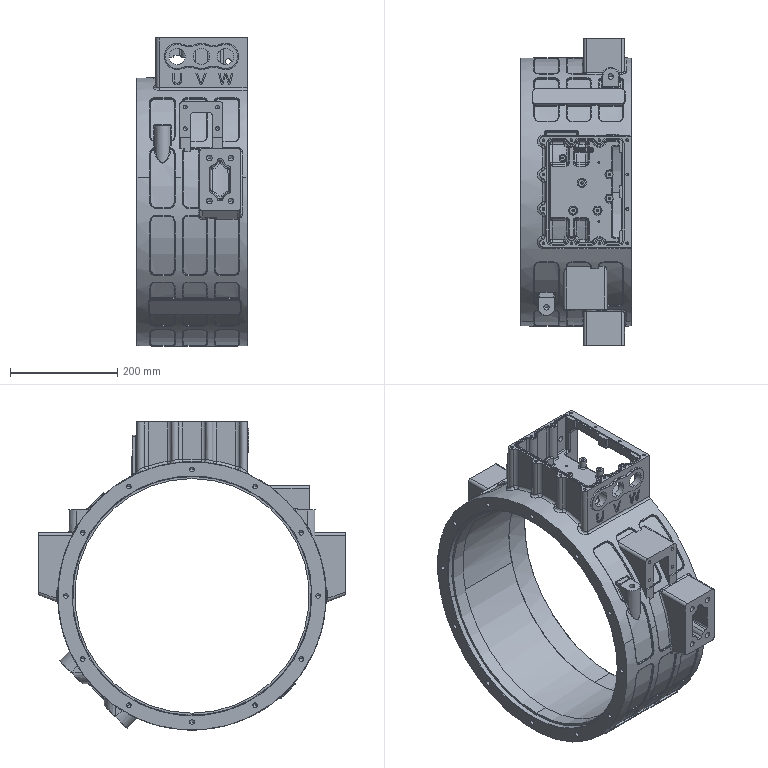Part | SolidWorks | features BaseBody 1 | 1 solid | 2181 faces | box 205 x 571.5 x 574 mm | volume 7765718 mm3 | cylinder 750 | spline 528 | plane 301 | torus 291 | cone 191 | sphere 120 | commonest cylinder face diameters 2 x177 20 x115 4 x83 8.5 x52 10 x51 5 x46